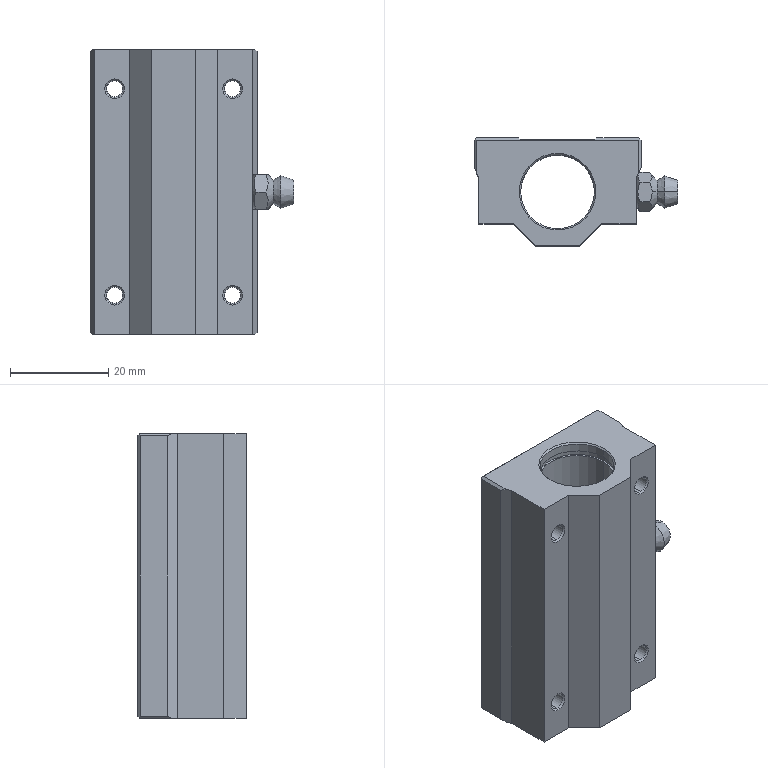Part | SolidWorks | features MBimport 1 | 1 solid | 105 faces | box 41.5 x 22 x 58 mm | volume 25731 mm3 | plane 46 | cylinder 31 | cone 28 | commonest cylinder face diameters 3.242 x8 3.4 x8 15 x6 3 x4 15.8 x4 10 x1